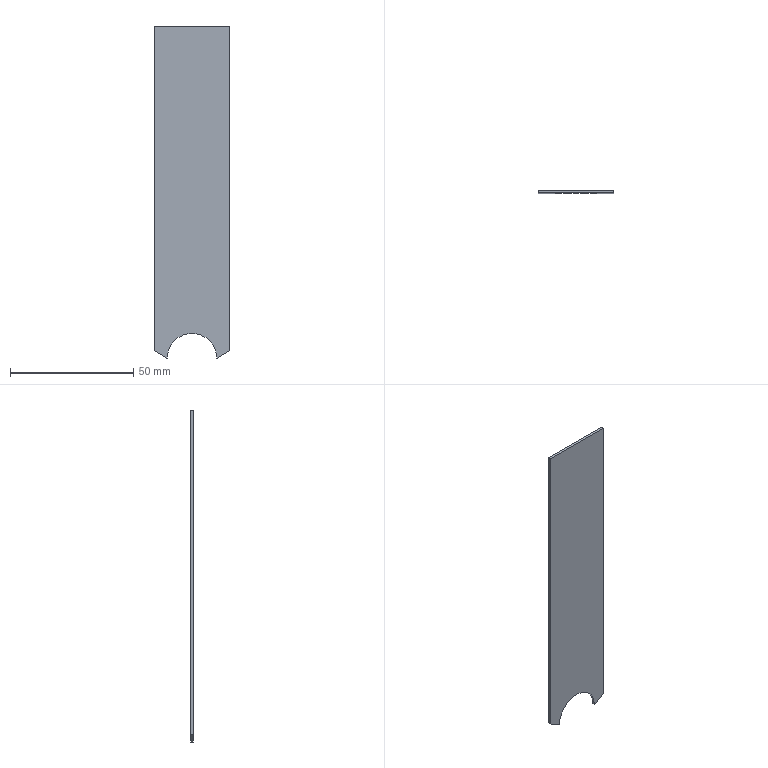Part | STEP file | solid 165 | 1 solid | 10 faces | box 30.5 x 1 x 134.425 mm | volume 3931 mm3 | plane 5 | cylinder 3 | cone 2 | commonest cylinder face diameters 30.5 x2 20 x1